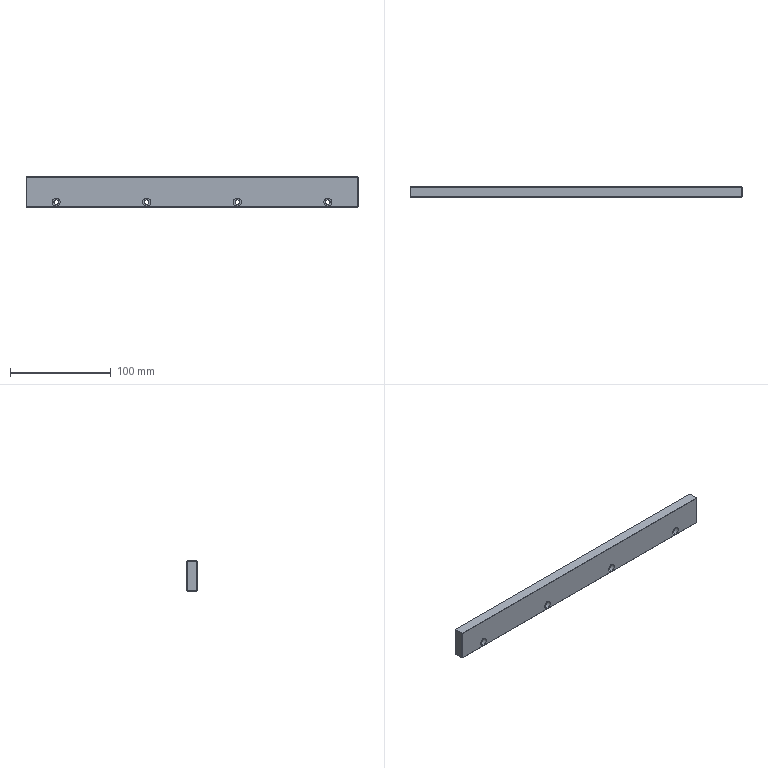Part | SolidWorks | features Chamfer 1, Extrusion 1, HoleWzd 1 | 1 solid | 46 faces | box 330 x 10 x 30 mm | volume 97693 mm3 | plane 30 | cylinder 16 | commonest cylinder face diameters 4.5 x8 8 x8
STEP:
#1=CARTESIAN_POINT('',(135.,4.4,-6.));
#2=VERTEX_POINT('',#1);
#3=CARTESIAN_POINT('',(135.,4.4,-14.));
#4=VERTEX_POINT('',#3);
#5=CARTESIAN_POINT('',(135.,4.4,-10.));
#6=DIRECTION('',(0.,-1.,0.));
#7=DIRECTION('',(0.,0.,-1.));
#8=AXIS2_PLACEMENT_3D('',#5,#6,#7);
#9=CIRCLE('',#8,4.);
#10=EDGE_CURVE('',#2,#4,#9,.T.);
#11=ORIENTED_EDGE('',*,*,#10,.F.);
#12=CARTESIAN_POINT('',(135.,0.,-6.));
#13=VERTEX_POINT('',#12);
#14=CARTESIAN_POINT('',(135.,0.,-6.));
#15=DIRECTION('',(0.,-1.,0.));
#16=VECTOR('',#15,1000.);
#17=LINE('',#14,#16);
#18=EDGE_CURVE('',#2,#13,#17,.T.);
#19=ORIENTED_EDGE('',*,*,#18,.T.);
#20=CARTESIAN_POINT('',(135.,0.,-14.));
#21=VERTEX_POINT('',#20);
#22=CARTESIAN_POINT('',(135.,0.,-10.));
#23=DIRECTION('',(0.,-1.,0.));
#24=DIRECTION('',(0.,0.,-1.));
#25=AXIS2_PLACEMENT_3D('',#22,#23,#24);
#26=CIRCLE('',#25,4.);
#27=EDGE_CURVE('',#13,#21,#26,.T.);
#28=ORIENTED_EDGE('',*,*,#27,.T.);
#29=CARTESIAN_POINT('',(135.,0.,-14.));
#30=DIRECTION('',(0.,-1.,0.));
#31=VECTOR('',#30,1000.);
#32=LINE('',#29,#31);
#33=EDGE_CURVE('',#4,#21,#32,.T.);
#34=ORIENTED_EDGE('',*,*,#33,.F.);
#35=EDGE_LOOP('',(#11,#19,#28,#34));
#36=FACE_OUTER_BOUND('',#35,.T.);
#37=CARTESIAN_POINT('',(135.,0.,-10.));
#38=DIRECTION('',(0.,-1.,0.));
#39=DIRECTION('',(0.,0.,-1.));
#40=AXIS2_PLACEMENT_3D('',#37,#38,#39);
#41=CYLINDRICAL_SURFACE('',#40,4.);
#42=ADVANCED_FACE('',(#36),#41,.F.);
#43=CARTESIAN_POINT('',(135.,10.,-7.75));
#44=VERTEX_POINT('',#43);
#45=CARTESIAN_POINT('',(135.,10.,-12.25));
#46=VERTEX_POINT('',#45);
#47=CARTESIAN_POINT('',(135.,10.,-10.));
#48=DIRECTION('',(0.,-1.,0.));
#49=DIRECTION('',(0.,0.,-1.));
#50=AXIS2_PLACEMENT_3D('',#47,#48,#49);
#51=CIRCLE('',#50,2.25);
#52=EDGE_CURVE('',#44,#46,#51,.T.);
#53=ORIENTED_EDGE('',*,*,#52,.F.);
#54=CARTESIAN_POINT('',(135.,4.4,-7.75));
#55=VERTEX_POINT('',#54);
#56=CARTESIAN_POINT('',(135.,0.,-7.75));
#57=DIRECTION('',(0.,-1.,0.));
#58=VECTOR('',#57,1000.);
#59=LINE('',#56,#58);
#60=EDGE_CURVE('',#44,#55,#59,.T.);
#61=ORIENTED_EDGE('',*,*,#60,.T.);
#62=CARTESIAN_POINT('',(135.,4.4,-12.25));
#63=VERTEX_POINT('',#62);
#64=CARTESIAN_POINT('',(135.,4.4,-10.));
#65=DIRECTION('',(0.,-1.,0.));
#66=DIRECTION('',(0.,0.,-1.));
#67=AXIS2_PLACEMENT_3D('',#64,#65,#66);
#68=CIRCLE('',#67,2.25);
#69=EDGE_CURVE('',#55,#63,#68,.T.);
#70=ORIENTED_EDGE('',*,*,#69,.T.);
#71=CARTESIAN_POINT('',(135.,0.,-12.25));
#72=DIRECTION('',(0.,-1.,0.));
#73=VECTOR('',#72,1000.);
#74=LINE('',#71,#73);
#75=EDGE_CURVE('',#46,#63,#74,.T.);
#76=ORIENTED_EDGE('',*,*,#75,.F.);
#77=EDGE_LOOP('',(#53,#61,#70,#76));
#78=FACE_OUTER_BOUND('',#77,.T.);
#79=CARTESIAN_POINT('',(135.,0.,-10.));
#80=DIRECTION('',(0.,-1.,0.));
#81=DIRECTION('',(0.,0.,-1.));
#82=AXIS2_PLACEMENT_3D('',#79,#80,#81);
#83=CYLINDRICAL_SURFACE('',#82,2.25);
#84=ADVANCED_FACE('',(#78),#83,.F.);
#85=CARTESIAN_POINT('',(45.,4.4,-6.));
#86=VERTEX_POINT('',#85);
#87=CARTESIAN_POINT('',(45.,4.4,-14.));
#88=VERTEX_POINT('',#87);
#89=CARTESIAN_POINT('',(45.,4.4,-10.));
#90=DIRECTION('',(0.,-1.,0.));
#91=DIRECTION('',(0.,0.,-1.));
#92=AXIS2_PLACEMENT_3D('',#89,#90,#91);
#93=CIRCLE('',#92,4.);
#94=EDGE_CURVE('',#86,#88,#93,.T.);
#95=ORIENTED_EDGE('',*,*,#94,.F.);
#96=CARTESIAN_POINT('',(45.,0.,-6.));
#97=VERTEX_POINT('',#96);
#98=CARTESIAN_POINT('',(45.,0.,-6.));
#99=DIRECTION('',(0.,-1.,0.));
#100=VECTOR('',#99,1000.);
#101=LINE('',#98,#100);
#102=EDGE_CURVE('',#86,#97,#101,.T.);
#103=ORIENTED_EDGE('',*,*,#102,.T.);
#104=CARTESIAN_POINT('',(45.,0.,-14.));
#105=VERTEX_POINT('',#104);
#106=CARTESIAN_POINT('',(45.,0.,-10.));
#107=DIRECTION('',(0.,-1.,0.));
#108=DIRECTION('',(0.,0.,-1.));
#109=AXIS2_PLACEMENT_3D('',#106,#107,#108);
#110=CIRCLE('',#109,4.);
#111=EDGE_CURVE('',#97,#105,#110,.T.);
#112=ORIENTED_EDGE('',*,*,#111,.T.);
#113=CARTESIAN_POINT('',(45.,0.,-14.));
#114=DIRECTION('',(0.,-1.,0.));
#115=VECTOR('',#114,1000.);
#116=LINE('',#113,#115);
#117=EDGE_CURVE('',#88,#105,#116,.T.);
#118=ORIENTED_EDGE('',*,*,#117,.F.);
#119=EDGE_LOOP('',(#95,#103,#112,#118));
#120=FACE_OUTER_BOUND('',#119,.T.);
#121=CARTESIAN_POINT('',(45.,0.,-10.));
#122=DIRECTION('',(0.,-1.,0.));
#123=DIRECTION('',(0.,0.,-1.));
#124=AXIS2_PLACEMENT_3D('',#121,#122,#123);
#125=CYLINDRICAL_SURFACE('',#124,4.);
#126=ADVANCED_FACE('',(#120),#125,.F.);
#127=CARTESIAN_POINT('',(45.,10.,-7.75));
#128=VERTEX_POINT('',#127);
#129=CARTESIAN_POINT('',(45.,10.,-12.25));
#130=VERTEX_POINT('',#129);
#131=CARTESIAN_POINT('',(45.,10.,-10.));
#132=DIRECTION('',(0.,-1.,0.));
#133=DIRECTION('',(0.,0.,-1.));
#134=AXIS2_PLACEMENT_3D('',#131,#132,#133);
#135=CIRCLE('',#134,2.25);
#136=EDGE_CURVE('',#128,#130,#135,.T.);
#137=ORIENTED_EDGE('',*,*,#136,.F.);
#138=CARTESIAN_POINT('',(45.,4.4,-7.75));
#139=VERTEX_POINT('',#138);
#140=CARTESIAN_POINT('',(45.,0.,-7.75));
#141=DIRECTION('',(0.,-1.,0.));
#142=VECTOR('',#141,1000.);
#143=LINE('',#140,#142);
#144=EDGE_CURVE('',#128,#139,#143,.T.);
#145=ORIENTED_EDGE('',*,*,#144,.T.);
#146=CARTESIAN_POINT('',(45.,4.4,-12.25));
#147=VERTEX_POINT('',#146);
#148=CARTESIAN_POINT('',(45.,4.4,-10.));
#149=DIRECTION('',(0.,-1.,0.));
#150=DIRECTION('',(0.,0.,-1.));
#151=AXIS2_PLACEMENT_3D('',#148,#149,#150);
#152=CIRCLE('',#151,2.25);
#153=EDGE_CURVE('',#139,#147,#152,.T.);
#154=ORIENTED_EDGE('',*,*,#153,.T.);
#155=CARTESIAN_POINT('',(45.,0.,-12.25));
#156=DIRECTION('',(0.,-1.,0.));
#157=VECTOR('',#156,1000.);
#158=LINE('',#155,#157);
#159=EDGE_CURVE('',#130,#147,#158,.T.);
#160=ORIENTED_EDGE('',*,*,#159,.F.);
#161=EDGE_LOOP('',(#137,#145,#154,#160));
#162=FACE_OUTER_BOUND('',#161,.T.);
#163=CARTESIAN_POINT('',(45.,0.,-10.));
#164=DIRECTION('',(0.,-1.,0.));
#165=DIRECTION('',(0.,0.,-1.));
#166=AXIS2_PLACEMENT_3D('',#163,#164,#165);
#167=CYLINDRICAL_SURFACE('',#166,2.25);
#168=ADVANCED_FACE('',(#162),#167,.F.);
#169=CARTESIAN_POINT('',(-45.,4.4,-6.));
#170=VERTEX_POINT('',#169);
#171=CARTESIAN_POINT('',(-45.,4.4,-14.));
#172=VERTEX_POINT('',#171);
#173=CARTESIAN_POINT('',(-45.,4.4,-10.));
#174=DIRECTION('',(0.,-1.,0.));
#175=DIRECTION('',(0.,0.,-1.));
#176=AXIS2_PLACEMENT_3D('',#173,#174,#175);
#177=CIRCLE('',#176,4.);
#178=EDGE_CURVE('',#170,#172,#177,.T.);
#179=ORIENTED_EDGE('',*,*,#178,.F.);
#180=CARTESIAN_POINT('',(-45.,0.,-6.));
#181=VERTEX_POINT('',#180);
#182=CARTESIAN_POINT('',(-45.,0.,-6.));
#183=DIRECTION('',(0.,-1.,0.));
#184=VECTOR('',#183,1000.);
#185=LINE('',#182,#184);
#186=EDGE_CURVE('',#170,#181,#185,.T.);
#187=ORIENTED_EDGE('',*,*,#186,.T.);
#188=CARTESIAN_POINT('',(-45.,0.,-14.));
#189=VERTEX_POINT('',#188);
#190=CARTESIAN_POINT('',(-45.,0.,-10.));
#191=DIRECTION('',(0.,-1.,0.));
#192=DIRECTION('',(0.,0.,-1.));
#193=AXIS2_PLACEMENT_3D('',#190,#191,#192);
#194=CIRCLE('',#193,4.);
#195=EDGE_CURVE('',#181,#189,#194,.T.);
#196=ORIENTED_EDGE('',*,*,#195,.T.);
#197=CARTESIAN_POINT('',(-45.,0.,-14.));
#198=DIRECTION('',(0.,-1.,0.));
#199=VECTOR('',#198,1000.);
#200=LINE('',#197,#199);
#201=EDGE_CURVE('',#172,#189,#200,.T.);
#202=ORIENTED_EDGE('',*,*,#201,.F.);
#203=EDGE_LOOP('',(#179,#187,#196,#202));
#204=FACE_OUTER_BOUND('',#203,.T.);
#205=CARTESIAN_POINT('',(-45.,0.,-10.));
#206=DIRECTION('',(0.,-1.,0.));
#207=DIRECTION('',(0.,0.,-1.));
#208=AXIS2_PLACEMENT_3D('',#205,#206,#207);
#209=CYLINDRICAL_SURFACE('',#208,4.);
#210=ADVANCED_FACE('',(#204),#209,.F.);
#211=CARTESIAN_POINT('',(-45.,10.,-7.75));
#212=VERTEX_POINT('',#211);
#213=CARTESIAN_POINT('',(-45.,10.,-12.25));
#214=VERTEX_POINT('',#213);
#215=CARTESIAN_POINT('',(-45.,10.,-10.));
#216=DIRECTION('',(0.,-1.,0.));
#217=DIRECTION('',(0.,0.,-1.));
#218=AXIS2_PLACEMENT_3D('',#215,#216,#217);
#219=CIRCLE('',#218,2.25);
#220=EDGE_CURVE('',#212,#214,#219,.T.);
#221=ORIENTED_EDGE('',*,*,#220,.F.);
#222=CARTESIAN_POINT('',(-45.,4.4,-7.75));
#223=VERTEX_POINT('',#222);
#224=CARTESIAN_POINT('',(-45.,0.,-7.75));
#225=DIRECTION('',(0.,-1.,0.));
#226=VECTOR('',#225,1000.);
#227=LINE('',#224,#226);
#228=EDGE_CURVE('',#212,#223,#227,.T.);
#229=ORIENTED_EDGE('',*,*,#228,.T.);
#230=CARTESIAN_POINT('',(-45.,4.4,-12.25));
#231=VERTEX_POINT('',#230);
#232=CARTESIAN_POINT('',(-45.,4.4,-10.));
#233=DIRECTION('',(0.,-1.,0.));
#234=DIRECTION('',(0.,0.,-1.));
#235=AXIS2_PLACEMENT_3D('',#232,#233,#234);
#236=CIRCLE('',#235,2.25);
#237=EDGE_CURVE('',#223,#231,#236,.T.);
#238=ORIENTED_EDGE('',*,*,#237,.T.);
#239=CARTESIAN_POINT('',(-45.,0.,-12.25));
#240=DIRECTION('',(0.,-1.,0.));
#241=VECTOR('',#240,1000.);
#242=LINE('',#239,#241);
#243=EDGE_CURVE('',#214,#231,#242,.T.);
#244=ORIENTED_EDGE('',*,*,#243,.F.);
#245=EDGE_LOOP('',(#221,#229,#238,#244));
#246=FACE_OUTER_BOUND('',#245,.T.);
#247=CARTESIAN_POINT('',(-45.,0.,-10.));
#248=DIRECTION('',(0.,-1.,0.));
#249=DIRECTION('',(0.,0.,-1.));
#250=AXIS2_PLACEMENT_3D('',#247,#248,#249);
#251=CYLINDRICAL_SURFACE('',#250,2.25);
#252=ADVANCED_FACE('',(#246),#251,.F.);
#253=CARTESIAN_POINT('',(-135.,4.4,-6.));
#254=VERTEX_POINT('',#253);
#255=CARTESIAN_POINT('',(-135.,4.4,-14.));
#256=VERTEX_POINT('',#255);
#257=CARTESIAN_POINT('',(-135.,4.4,-10.));
#258=DIRECTION('',(0.,-1.,0.));
#259=DIRECTION('',(0.,0.,-1.));
#260=AXIS2_PLACEMENT_3D('',#257,#258,#259);
#261=CIRCLE('',#260,4.);
#262=EDGE_CURVE('',#254,#256,#261,.T.);
#263=ORIENTED_EDGE('',*,*,#262,.F.);
#264=CARTESIAN_POINT('',(-135.,0.,-6.));
#265=VERTEX_POINT('',#264);
#266=CARTESIAN_POINT('',(-135.,0.,-6.));
#267=DIRECTION('',(0.,-1.,0.));
#268=VECTOR('',#267,1000.);
#269=LINE('',#266,#268);
#270=EDGE_CURVE('',#254,#265,#269,.T.);
#271=ORIENTED_EDGE('',*,*,#270,.T.);
#272=CARTESIAN_POINT('',(-135.,0.,-14.));
#273=VERTEX_POINT('',#272);
#274=CARTESIAN_POINT('',(-135.,0.,-10.));
#275=DIRECTION('',(0.,-1.,0.));
#276=DIRECTION('',(0.,0.,-1.));
#277=AXIS2_PLACEMENT_3D('',#274,#275,#276);
#278=CIRCLE('',#277,4.);
#279=EDGE_CURVE('',#265,#273,#278,.T.);
#280=ORIENTED_EDGE('',*,*,#279,.T.);
#281=CARTESIAN_POINT('',(-135.,0.,-14.));
#282=DIRECTION('',(0.,-1.,0.));
#283=VECTOR('',#282,1000.);
#284=LINE('',#281,#283);
#285=EDGE_CURVE('',#256,#273,#284,.T.);
#286=ORIENTED_EDGE('',*,*,#285,.F.);
#287=EDGE_LOOP('',(#263,#271,#280,#286));
#288=FACE_OUTER_BOUND('',#287,.T.);
#289=CARTESIAN_POINT('',(-135.,0.,-10.));
#290=DIRECTION('',(0.,-1.,0.));
#291=DIRECTION('',(0.,0.,-1.));
#292=AXIS2_PLACEMENT_3D('',#289,#290,#291);
#293=CYLINDRICAL_SURFACE('',#292,4.);
#294=ADVANCED_FACE('',(#288),#293,.F.);
#295=CARTESIAN_POINT('',(-135.,10.,-7.75));
#296=VERTEX_POINT('',#295);
#297=CARTESIAN_POINT('',(-135.,10.,-12.25));
#298=VERTEX_POINT('',#297);
#299=CARTESIAN_POINT('',(-135.,10.,-10.));
#300=DIRECTION('',(0.,-1.,0.));
#301=DIRECTION('',(0.,0.,-1.));
#302=AXIS2_PLACEMENT_3D('',#299,#300,#301);
#303=CIRCLE('',#302,2.25);
#304=EDGE_CURVE('',#296,#298,#303,.T.);
#305=ORIENTED_EDGE('',*,*,#304,.F.);
#306=CARTESIAN_POINT('',(-135.,4.4,-7.75));
#307=VERTEX_POINT('',#306);
#308=CARTESIAN_POINT('',(-135.,0.,-7.75));
#309=DIRECTION('',(0.,-1.,0.));
#310=VECTOR('',#309,1000.);
#311=LINE('',#308,#310);
#312=EDGE_CURVE('',#296,#307,#311,.T.);
#313=ORIENTED_EDGE('',*,*,#312,.T.);
#314=CARTESIAN_POINT('',(-135.,4.4,-12.25));
#315=VERTEX_POINT('',#314);
#316=CARTESIAN_POINT('',(-135.,4.4,-10.));
#317=DIRECTION('',(0.,-1.,0.));
#318=DIRECTION('',(0.,0.,-1.));
#319=AXIS2_PLACEMENT_3D('',#316,#317,#318);
#320=CIRCLE('',#319,2.25);
#321=EDGE_CURVE('',#307,#315,#320,.T.);
#322=ORIENTED_EDGE('',*,*,#321,.T.);
#323=CARTESIAN_POINT('',(-135.,0.,-12.25));
#324=DIRECTION('',(0.,-1.,0.));
#325=VECTOR('',#324,1000.);
#326=LINE('',#323,#325);
#327=EDGE_CURVE('',#298,#315,#326,.T.);
#328=ORIENTED_EDGE('',*,*,#327,.F.);
#329=EDGE_LOOP('',(#305,#313,#322,#328));
#330=FACE_OUTER_BOUND('',#329,.T.);
#331=CARTESIAN_POINT('',(-135.,0.,-10.));
#332=DIRECTION('',(0.,-1.,0.));
#333=DIRECTION('',(0.,0.,-1.));
#334=AXIS2_PLACEMENT_3D('',#331,#332,#333);
#335=CYLINDRICAL_SURFACE('',#334,2.25);
#336=ADVANCED_FACE('',(#330),#335,.F.);
#337=CARTESIAN_POINT('',(165.,9.7,-14.7));
#338=VERTEX_POINT('',#337);
#339=CARTESIAN_POINT('',(165.,9.7,14.7));
#340=VERTEX_POINT('',#339);
#341=CARTESIAN_POINT('',(165.,9.7,15.));
#342=DIRECTION('',(0.,0.,1.));
#343=VECTOR('',#342,1000.);
#344=LINE('',#341,#343);
#345=EDGE_CURVE('',#338,#340,#344,.T.);
#346=ORIENTED_EDGE('',*,*,#345,.T.);
#347=CARTESIAN_POINT('',(165.,0.3,14.7));
#348=VERTEX_POINT('',#347);
#349=CARTESIAN_POINT('',(165.,10.,14.7));
#350=DIRECTION('',(0.,-1.,0.));
#351=VECTOR('',#350,1000.);
#352=LINE('',#349,#351);
#353=EDGE_CURVE('',#340,#348,#352,.T.);
#354=ORIENTED_EDGE('',*,*,#353,.T.);
#355=CARTESIAN_POINT('',(165.,0.3,-14.7));
#356=VERTEX_POINT('',#355);
#357=CARTESIAN_POINT('',(165.,0.3,-15.));
#358=DIRECTION('',(0.,0.,-1.));
#359=VECTOR('',#358,1000.);
#360=LINE('',#357,#359);
#361=EDGE_CURVE('',#348,#356,#360,.T.);
#362=ORIENTED_EDGE('',*,*,#361,.T.);
#363=CARTESIAN_POINT('',(165.,10.,-14.7));
#364=DIRECTION('',(0.,1.,0.));
#365=VECTOR('',#364,1000.);
#366=LINE('',#363,#365);
#367=EDGE_CURVE('',#356,#338,#366,.T.);
#368=ORIENTED_EDGE('',*,*,#367,.T.);
#369=EDGE_LOOP('',(#346,#354,#362,#368));
#370=FACE_OUTER_BOUND('',#369,.T.);
#371=CARTESIAN_POINT('',(165.,10.,-15.));
#372=DIRECTION('',(-1.,0.,0.));
#373=DIRECTION('',(0.,0.,1.));
#374=AXIS2_PLACEMENT_3D('',#371,#372,#373);
#375=PLANE('',#374);
#376=ADVANCED_FACE('',(#370),#375,.F.);
#377=CARTESIAN_POINT('',(-164.7,9.7,-15.));
#378=VERTEX_POINT('',#377);
#379=CARTESIAN_POINT('',(164.7,9.7,-15.));
#380=VERTEX_POINT('',#379);
#381=CARTESIAN_POINT('',(165.,9.7,-15.));
#382=DIRECTION('',(1.,0.,0.));
#383=VECTOR('',#382,1000.);
#384=LINE('',#381,#383);
#385=EDGE_CURVE('',#378,#380,#384,.T.);
#386=ORIENTED_EDGE('',*,*,#385,.T.);
#387=CARTESIAN_POINT('',(164.7,0.3,-15.));
#388=VERTEX_POINT('',#387);
#389=CARTESIAN_POINT('',(164.7,10.,-15.));
#390=DIRECTION('',(0.,-1.,0.));
#391=VECTOR('',#390,1000.);
#392=LINE('',#389,#391);
#393=EDGE_CURVE('',#380,#388,#392,.T.);
#394=ORIENTED_EDGE('',*,*,#393,.T.);
#395=CARTESIAN_POINT('',(-164.7,0.3,-15.));
#396=VERTEX_POINT('',#395);
#397=CARTESIAN_POINT('',(-165.,0.3,-15.));
#398=DIRECTION('',(-1.,0.,0.));
#399=VECTOR('',#398,1000.);
#400=LINE('',#397,#399);
#401=EDGE_CURVE('',#388,#396,#400,.T.);
#402=ORIENTED_EDGE('',*,*,#401,.T.);
#403=CARTESIAN_POINT('',(-164.7,10.,-15.));
#404=DIRECTION('',(0.,1.,0.));
#405=VECTOR('',#404,1000.);
#406=LINE('',#403,#405);
#407=EDGE_CURVE('',#396,#378,#406,.T.);
#408=ORIENTED_EDGE('',*,*,#407,.T.);
#409=EDGE_LOOP('',(#386,#394,#402,#408));
#410=FACE_OUTER_BOUND('',#409,.T.);
#411=CARTESIAN_POINT('',(-165.,10.,-15.));
#412=DIRECTION('',(0.,0.,1.));
#413=DIRECTION('',(1.,0.,0.));
#414=AXIS2_PLACEMENT_3D('',#411,#412,#413);
#415=PLANE('',#414);
#416=ADVANCED_FACE('',(#410),#415,.F.);
#417=CARTESIAN_POINT('',(-165.,0.3,14.7));
#418=VERTEX_POINT('',#417);
#419=CARTESIAN_POINT('',(-165.,9.7,14.7));
#420=VERTEX_POINT('',#419);
#421=CARTESIAN_POINT('',(-165.,10.,14.7));
#422=DIRECTION('',(0.,1.,0.));
#423=VECTOR('',#422,1000.);
#424=LINE('',#421,#423);
#425=EDGE_CURVE('',#418,#420,#424,.T.);
#426=ORIENTED_EDGE('',*,*,#425,.T.);
#427=CARTESIAN_POINT('',(-165.,9.7,-14.7));
#428=VERTEX_POINT('',#427);
#429=CARTESIAN_POINT('',(-165.,9.7,-15.));
#430=DIRECTION('',(0.,0.,-1.));
#431=VECTOR('',#430,1000.);
#432=LINE('',#429,#431);
#433=EDGE_CURVE('',#420,#428,#432,.T.);
#434=ORIENTED_EDGE('',*,*,#433,.T.);
#435=CARTESIAN_POINT('',(-165.,0.3,-14.7));
#436=VERTEX_POINT('',#435);
#437=CARTESIAN_POINT('',(-165.,10.,-14.7));
#438=DIRECTION('',(0.,-1.,0.));
#439=VECTOR('',#438,1000.);
#440=LINE('',#437,#439);
#441=EDGE_CURVE('',#428,#436,#440,.T.);
#442=ORIENTED_EDGE('',*,*,#441,.T.);
#443=CARTESIAN_POINT('',(-165.,0.3,-15.));
#444=DIRECTION('',(0.,0.,1.));
#445=VECTOR('',#444,1000.);
#446=LINE('',#443,#445);
#447=EDGE_CURVE('',#436,#418,#446,.T.);
#448=ORIENTED_EDGE('',*,*,#447,.T.);
#449=EDGE_LOOP('',(#426,#434,#442,#448));
#450=FACE_OUTER_BOUND('',#449,.T.);
#451=CARTESIAN_POINT('',(-165.,10.,-15.));
#452=DIRECTION('',(1.,0.,0.));
#453=DIRECTION('',(0.,0.,-1.));
#454=AXIS2_PLACEMENT_3D('',#451,#452,#453);
#455=PLANE('',#454);
#456=ADVANCED_FACE('',(#450),#455,.F.);
#457=CARTESIAN_POINT('',(164.7,0.3,15.));
#458=VERTEX_POINT('',#457);
#459=CARTESIAN_POINT('',(164.7,9.7,15.));
#460=VERTEX_POINT('',#459);
#461=CARTESIAN_POINT('',(164.7,10.,15.));
#462=DIRECTION('',(0.,1.,0.));
#463=VECTOR('',#462,1000.);
#464=LINE('',#461,#463);
#465=EDGE_CURVE('',#458,#460,#464,.T.);
#466=ORIENTED_EDGE('',*,*,#465,.T.);
#467=CARTESIAN_POINT('',(-164.7,9.7,15.));
#468=VERTEX_POINT('',#467);
#469=CARTESIAN_POINT('',(-165.,9.7,15.));
#470=DIRECTION('',(-1.,0.,0.));
#471=VECTOR('',#470,1000.);
#472=LINE('',#469,#471);
#473=EDGE_CURVE('',#460,#468,#472,.T.);
#474=ORIENTED_EDGE('',*,*,#473,.T.);
#475=CARTESIAN_POINT('',(-164.7,0.3,15.));
#476=VERTEX_POINT('',#475);
#477=CARTESIAN_POINT('',(-164.7,10.,15.));
#478=DIRECTION('',(0.,-1.,0.));
#479=VECTOR('',#478,1000.);
#480=LINE('',#477,#479);
#481=EDGE_CURVE('',#468,#476,#480,.T.);
#482=ORIENTED_EDGE('',*,*,#481,.T.);
#483=CARTESIAN_POINT('',(-165.,0.3,15.));
#484=DIRECTION('',(1.,0.,0.));
#485=VECTOR('',#484,1000.);
#486=LINE('',#483,#485);
#487=EDGE_CURVE('',#476,#458,#486,.T.);
#488=ORIENTED_EDGE('',*,*,#487,.T.);
#489=EDGE_LOOP('',(#466,#474,#482,#488));
#490=FACE_OUTER_BOUND('',#489,.T.);
#491=CARTESIAN_POINT('',(-165.,10.,15.));
#492=DIRECTION('',(0.,0.,-1.));
#493=DIRECTION('',(-1.,0.,0.));
#494=AXIS2_PLACEMENT_3D('',#491,#492,#493);
#495=PLANE('',#494);
#496=ADVANCED_FACE('',(#490),#495,.F.);
#497=CARTESIAN_POINT('',(-164.7,10.,14.7));
#498=VERTEX_POINT('',#497);
#499=CARTESIAN_POINT('',(164.7,10.,14.7));
#500=VERTEX_POINT('',#499);
#501=CARTESIAN_POINT('',(165.,10.,14.7));
#502=DIRECTION('',(1.,0.,0.));
#503=VECTOR('',#502,1000.);
#504=LINE('',#501,#503);
#505=EDGE_CURVE('',#498,#500,#504,.T.);
#506=ORIENTED_EDGE('',*,*,#505,.T.);
#507=CARTESIAN_POINT('',(164.7,10.,-14.7));
#508=VERTEX_POINT('',#507);
#509=CARTESIAN_POINT('',(164.7,10.,-15.));
#510=DIRECTION('',(0.,0.,-1.));
#511=VECTOR('',#510,1000.);
#512=LINE('',#509,#511);
#513=EDGE_CURVE('',#500,#508,#512,.T.);
#514=ORIENTED_EDGE('',*,*,#513,.T.);
#515=CARTESIAN_POINT('',(-164.7,10.,-14.7));
#516=VERTEX_POINT('',#515);
#517=CARTESIAN_POINT('',(-165.,10.,-14.7));
#518=DIRECTION('',(-1.,0.,0.));
#519=VECTOR('',#518,1000.);
#520=LINE('',#517,#519);
#521=EDGE_CURVE('',#508,#516,#520,.T.);
#522=ORIENTED_EDGE('',*,*,#521,.T.);
#523=CARTESIAN_POINT('',(-164.7,10.,15.));
#524=DIRECTION('',(0.,0.,1.));
#525=VECTOR('',#524,1000.);
#526=LINE('',#523,#525);
#527=EDGE_CURVE('',#516,#498,#526,.T.);
#528=ORIENTED_EDGE('',*,*,#527,.T.);
#529=EDGE_LOOP('',(#506,#514,#522,#528));
#530=FACE_OUTER_BOUND('',#529,.T.);
#531=CARTESIAN_POINT('',(135.,10.,-10.));
#532=DIRECTION('',(0.,-1.,0.));
#533=DIRECTION('',(0.,0.,-1.));
#534=AXIS2_PLACEMENT_3D('',#531,#532,#533);
#535=CIRCLE('',#534,2.25);
#536=EDGE_CURVE('',#46,#44,#535,.T.);
#537=ORIENTED_EDGE('',*,*,#536,.T.);
#538=ORIENTED_EDGE('',*,*,#52,.T.);
#539=EDGE_LOOP('',(#537,#538));
#540=FACE_BOUND('',#539,.T.);
#541=CARTESIAN_POINT('',(45.,10.,-10.));
#542=DIRECTION('',(0.,-1.,0.));
#543=DIRECTION('',(0.,0.,-1.));
#544=AXIS2_PLACEMENT_3D('',#541,#542,#543);
#545=CIRCLE('',#544,2.25);
#546=EDGE_CURVE('',#130,#128,#545,.T.);
#547=ORIENTED_EDGE('',*,*,#546,.T.);
#548=ORIENTED_EDGE('',*,*,#136,.T.);
#549=EDGE_LOOP('',(#547,#548));
#550=FACE_BOUND('',#549,.T.);
#551=CARTESIAN_POINT('',(-45.,10.,-10.));
#552=DIRECTION('',(0.,-1.,0.));
#553=DIRECTION('',(0.,0.,-1.));
#554=AXIS2_PLACEMENT_3D('',#551,#552,#553);
#555=CIRCLE('',#554,2.25);
#556=EDGE_CURVE('',#214,#212,#555,.T.);
#557=ORIENTED_EDGE('',*,*,#556,.T.);
#558=ORIENTED_EDGE('',*,*,#220,.T.);
#559=EDGE_LOOP('',(#557,#558));
#560=FACE_BOUND('',#559,.T.);
#561=CARTESIAN_POINT('',(-135.,10.,-10.));
#562=DIRECTION('',(0.,-1.,0.));
#563=DIRECTION('',(0.,0.,-1.));
#564=AXIS2_PLACEMENT_3D('',#561,#562,#563);
#565=CIRCLE('',#564,2.25);
#566=EDGE_CURVE('',#298,#296,#565,.T.);
#567=ORIENTED_EDGE('',*,*,#566,.T.);
#568=ORIENTED_EDGE('',*,*,#304,.T.);
#569=EDGE_LOOP('',(#567,#568));
#570=FACE_BOUND('',#569,.T.);
#571=CARTESIAN_POINT('',(0.,10.,0.));
#572=DIRECTION('',(0.,1.,0.));
#573=DIRECTION('',(0.,0.,1.));
#574=AXIS2_PLACEMENT_3D('',#571,#572,#573);
#575=PLANE('',#574);
#576=ADVANCED_FACE('',(#530,#540,#550,#560,#570),#575,.T.);
#577=CARTESIAN_POINT('',(-164.7,0.,-14.7));
#578=VERTEX_POINT('',#577);
#579=CARTESIAN_POINT('',(164.7,0.,-14.7));
#580=VERTEX_POINT('',#579);
#581=CARTESIAN_POINT('',(0.,0.,-14.7));
#582=DIRECTION('',(1.,0.,0.));
#583=VECTOR('',#582,1000.);
#584=LINE('',#581,#583);
#585=EDGE_CURVE('',#578,#580,#584,.T.);
#586=ORIENTED_EDGE('',*,*,#585,.T.);
#587=CARTESIAN_POINT('',(164.7,0.,14.7));
#588=VERTEX_POINT('',#587);
#589=CARTESIAN_POINT('',(164.7,0.,0.));
#590=DIRECTION('',(0.,0.,1.));
#591=VECTOR('',#590,1000.);
#592=LINE('',#589,#591);
#593=EDGE_CURVE('',#580,#588,#592,.T.);
#594=ORIENTED_EDGE('',*,*,#593,.T.);
#595=CARTESIAN_POINT('',(-164.7,0.,14.7));
#596=VERTEX_POINT('',#595);
#597=CARTESIAN_POINT('',(0.,0.,14.7));
#598=DIRECTION('',(-1.,0.,0.));
#599=VECTOR('',#598,1000.);
#600=LINE('',#597,#599);
#601=EDGE_CURVE('',#588,#596,#600,.T.);
#602=ORIENTED_EDGE('',*,*,#601,.T.);
#603=CARTESIAN_POINT('',(-164.7,0.,0.));
#604=DIRECTION('',(0.,0.,-1.));
#605=VECTOR('',#604,1000.);
#606=LINE('',#603,#605);
#607=EDGE_CURVE('',#596,#578,#606,.T.);
#608=ORIENTED_EDGE('',*,*,#607,.T.);
#609=EDGE_LOOP('',(#586,#594,#602,#608));
#610=FACE_OUTER_BOUND('',#609,.T.);
#611=CARTESIAN_POINT('',(135.,0.,-10.));
#612=DIRECTION('',(0.,-1.,0.));
#613=DIRECTION('',(0.,0.,-1.));
#614=AXIS2_PLACEMENT_3D('',#611,#612,#613);
#615=CIRCLE('',#614,4.);
#616=EDGE_CURVE('',#21,#13,#615,.T.);
#617=ORIENTED_EDGE('',*,*,#616,.F.);
#618=ORIENTED_EDGE('',*,*,#27,.F.);
#619=EDGE_LOOP('',(#617,#618));
#620=FACE_BOUND('',#619,.T.);
#621=CARTESIAN_POINT('',(45.,0.,-10.));
#622=DIRECTION('',(0.,-1.,0.));
#623=DIRECTION('',(0.,0.,-1.));
#624=AXIS2_PLACEMENT_3D('',#621,#622,#623);
#625=CIRCLE('',#624,4.);
#626=EDGE_CURVE('',#105,#97,#625,.T.);
#627=ORIENTED_EDGE('',*,*,#626,.F.);
#628=ORIENTED_EDGE('',*,*,#111,.F.);
#629=EDGE_LOOP('',(#627,#628));
#630=FACE_BOUND('',#629,.T.);
#631=CARTESIAN_POINT('',(-45.,0.,-10.));
#632=DIRECTION('',(0.,-1.,0.));
#633=DIRECTION('',(0.,0.,-1.));
#634=AXIS2_PLACEMENT_3D('',#631,#632,#633);
#635=CIRCLE('',#634,4.);
#636=EDGE_CURVE('',#189,#181,#635,.T.);
#637=ORIENTED_EDGE('',*,*,#636,.F.);
#638=ORIENTED_EDGE('',*,*,#195,.F.);
#639=EDGE_LOOP('',(#637,#638));
#640=FACE_BOUND('',#639,.T.);
#641=CARTESIAN_POINT('',(-135.,0.,-10.));
#642=DIRECTION('',(0.,-1.,0.));
#643=DIRECTION('',(0.,0.,-1.));
#644=AXIS2_PLACEMENT_3D('',#641,#642,#643);
#645=CIRCLE('',#644,4.);
#646=EDGE_CURVE('',#273,#265,#645,.T.);
#647=ORIENTED_EDGE('',*,*,#646,.F.);
#648=ORIENTED_EDGE('',*,*,#279,.F.);
#649=EDGE_LOOP('',(#647,#648));
#650=FACE_BOUND('',#649,.T.);
#651=CARTESIAN_POINT('',(0.,0.,0.));
#652=DIRECTION('',(0.,1.,0.));
#653=DIRECTION('',(0.,0.,1.));
#654=AXIS2_PLACEMENT_3D('',#651,#652,#653);
#655=PLANE('',#654);
#656=ADVANCED_FACE('',(#610,#620,#630,#640,#650),#655,.F.);
#657=ORIENTED_EDGE('',*,*,#312,.F.);
#658=ORIENTED_EDGE('',*,*,#566,.F.);
#659=ORIENTED_EDGE('',*,*,#327,.T.);
#660=CARTESIAN_POINT('',(-135.,4.4,-10.));
#661=DIRECTION('',(0.,-1.,0.));
#662=DIRECTION('',(0.,0.,-1.));
#663=AXIS2_PLACEMENT_3D('',#660,#661,#662);
#664=CIRCLE('',#663,2.25);
#665=EDGE_CURVE('',#315,#307,#664,.T.);
#666=ORIENTED_EDGE('',*,*,#665,.T.);
#667=EDGE_LOOP('',(#657,#658,#659,#666));
#668=FACE_OUTER_BOUND('',#667,.T.);
#669=CARTESIAN_POINT('',(-135.,0.,-10.));
#670=DIRECTION('',(0.,-1.,0.));
#671=DIRECTION('',(0.,0.,-1.));
#672=AXIS2_PLACEMENT_3D('',#669,#670,#671);
#673=CYLINDRICAL_SURFACE('',#672,2.25);
#674=ADVANCED_FACE('',(#668),#673,.F.);
#675=ORIENTED_EDGE('',*,*,#665,.F.);
#676=ORIENTED_EDGE('',*,*,#321,.F.);
#677=EDGE_LOOP('',(#675,#676));
#678=FACE_BOUND('',#677,.T.);
#679=CARTESIAN_POINT('',(-135.,4.4,-10.));
#680=DIRECTION('',(0.,-1.,0.));
#681=DIRECTION('',(0.,0.,-1.));
#682=AXIS2_PLACEMENT_3D('',#679,#680,#681);
#683=CIRCLE('',#682,4.);
#684=EDGE_CURVE('',#256,#254,#683,.T.);
#685=ORIENTED_EDGE('',*,*,#684,.T.);
#686=ORIENTED_EDGE('',*,*,#262,.T.);
#687=EDGE_LOOP('',(#685,#686));
#688=FACE_OUTER_BOUND('',#687,.T.);
#689=CARTESIAN_POINT('',(-132.75,4.4,-10.));
#690=DIRECTION('',(0.,1.,0.));
#691=DIRECTION('',(0.,0.,1.));
#692=AXIS2_PLACEMENT_3D('',#689,#690,#691);
#693=PLANE('',#692);
#694=ADVANCED_FACE('',(#678,#688),#693,.F.);
#695=ORIENTED_EDGE('',*,*,#270,.F.);
#696=ORIENTED_EDGE('',*,*,#684,.F.);
#697=ORIENTED_EDGE('',*,*,#285,.T.);
#698=ORIENTED_EDGE('',*,*,#646,.T.);
#699=EDGE_LOOP('',(#695,#696,#697,#698));
#700=FACE_OUTER_BOUND('',#699,.T.);
#701=CARTESIAN_POINT('',(-135.,0.,-10.));
#702=DIRECTION('',(0.,-1.,0.));
#703=DIRECTION('',(0.,0.,-1.));
#704=AXIS2_PLACEMENT_3D('',#701,#702,#703);
#705=CYLINDRICAL_SURFACE('',#704,4.);
#706=ADVANCED_FACE('',(#700),#705,.F.);
#707=ORIENTED_EDGE('',*,*,#228,.F.);
#708=ORIENTED_EDGE('',*,*,#556,.F.);
#709=ORIENTED_EDGE('',*,*,#243,.T.);
#710=CARTESIAN_POINT('',(-45.,4.4,-10.));
#711=DIRECTION('',(0.,-1.,0.));
#712=DIRECTION('',(0.,0.,-1.));
#713=AXIS2_PLACEMENT_3D('',#710,#711,#712);
#714=CIRCLE('',#713,2.25);
#715=EDGE_CURVE('',#231,#223,#714,.T.);
#716=ORIENTED_EDGE('',*,*,#715,.T.);
#717=EDGE_LOOP('',(#707,#708,#709,#716));
#718=FACE_OUTER_BOUND('',#717,.T.);
#719=CARTESIAN_POINT('',(-45.,0.,-10.));
#720=DIRECTION('',(0.,-1.,0.));
#721=DIRECTION('',(0.,0.,-1.));
#722=AXIS2_PLACEMENT_3D('',#719,#720,#721);
#723=CYLINDRICAL_SURFACE('',#722,2.25);
#724=ADVANCED_FACE('',(#718),#723,.F.);
#725=ORIENTED_EDGE('',*,*,#715,.F.);
#726=ORIENTED_EDGE('',*,*,#237,.F.);
#727=EDGE_LOOP('',(#725,#726));
#728=FACE_BOUND('',#727,.T.);
#729=CARTESIAN_POINT('',(-45.,4.4,-10.));
#730=DIRECTION('',(0.,-1.,0.));
#731=DIRECTION('',(0.,0.,-1.));
#732=AXIS2_PLACEMENT_3D('',#729,#730,#731);
#733=CIRCLE('',#732,4.);
#734=EDGE_CURVE('',#172,#170,#733,.T.);
#735=ORIENTED_EDGE('',*,*,#734,.T.);
#736=ORIENTED_EDGE('',*,*,#178,.T.);
#737=EDGE_LOOP('',(#735,#736));
#738=FACE_OUTER_BOUND('',#737,.T.);
#739=CARTESIAN_POINT('',(-42.75,4.4,-10.));
#740=DIRECTION('',(0.,1.,0.));
#741=DIRECTION('',(0.,0.,1.));
#742=AXIS2_PLACEMENT_3D('',#739,#740,#741);
#743=PLANE('',#742);
#744=ADVANCED_FACE('',(#728,#738),#743,.F.);
#745=ORIENTED_EDGE('',*,*,#186,.F.);
#746=ORIENTED_EDGE('',*,*,#734,.F.);
#747=ORIENTED_EDGE('',*,*,#201,.T.);
#748=ORIENTED_EDGE('',*,*,#636,.T.);
#749=EDGE_LOOP('',(#745,#746,#747,#748));
#750=FACE_OUTER_BOUND('',#749,.T.);
#751=CARTESIAN_POINT('',(-45.,0.,-10.));
#752=DIRECTION('',(0.,-1.,0.));
#753=DIRECTION('',(0.,0.,-1.));
#754=AXIS2_PLACEMENT_3D('',#751,#752,#753);
#755=CYLINDRICAL_SURFACE('',#754,4.);
#756=ADVANCED_FACE('',(#750),#755,.F.);
#757=ORIENTED_EDGE('',*,*,#144,.F.);
#758=ORIENTED_EDGE('',*,*,#546,.F.);
#759=ORIENTED_EDGE('',*,*,#159,.T.);
#760=CARTESIAN_POINT('',(45.,4.4,-10.));
#761=DIRECTION('',(0.,-1.,0.));
#762=DIRECTION('',(0.,0.,-1.));
#763=AXIS2_PLACEMENT_3D('',#760,#761,#762);
#764=CIRCLE('',#763,2.25);
#765=EDGE_CURVE('',#147,#139,#764,.T.);
#766=ORIENTED_EDGE('',*,*,#765,.T.);
#767=EDGE_LOOP('',(#757,#758,#759,#766));
#768=FACE_OUTER_BOUND('',#767,.T.);
#769=CARTESIAN_POINT('',(45.,0.,-10.));
#770=DIRECTION('',(0.,-1.,0.));
#771=DIRECTION('',(0.,0.,-1.));
#772=AXIS2_PLACEMENT_3D('',#769,#770,#771);
#773=CYLINDRICAL_SURFACE('',#772,2.25);
#774=ADVANCED_FACE('',(#768),#773,.F.);
#775=ORIENTED_EDGE('',*,*,#765,.F.);
#776=ORIENTED_EDGE('',*,*,#153,.F.);
#777=EDGE_LOOP('',(#775,#776));
#778=FACE_BOUND('',#777,.T.);
#779=CARTESIAN_POINT('',(45.,4.4,-10.));
#780=DIRECTION('',(0.,-1.,0.));
#781=DIRECTION('',(0.,0.,-1.));
#782=AXIS2_PLACEMENT_3D('',#779,#780,#781);
#783=CIRCLE('',#782,4.);
#784=EDGE_CURVE('',#88,#86,#783,.T.);
#785=ORIENTED_EDGE('',*,*,#784,.T.);
#786=ORIENTED_EDGE('',*,*,#94,.T.);
#787=EDGE_LOOP('',(#785,#786));
#788=FACE_OUTER_BOUND('',#787,.T.);
#789=CARTESIAN_POINT('',(47.25,4.4,-10.));
#790=DIRECTION('',(0.,1.,0.));
#791=DIRECTION('',(0.,0.,1.));
#792=AXIS2_PLACEMENT_3D('',#789,#790,#791);
#793=PLANE('',#792);
#794=ADVANCED_FACE('',(#778,#788),#793,.F.);
#795=ORIENTED_EDGE('',*,*,#102,.F.);
#796=ORIENTED_EDGE('',*,*,#784,.F.);
#797=ORIENTED_EDGE('',*,*,#117,.T.);
#798=ORIENTED_EDGE('',*,*,#626,.T.);
#799=EDGE_LOOP('',(#795,#796,#797,#798));
#800=FACE_OUTER_BOUND('',#799,.T.);
#801=CARTESIAN_POINT('',(45.,0.,-10.));
#802=DIRECTION('',(0.,-1.,0.));
#803=DIRECTION('',(0.,0.,-1.));
#804=AXIS2_PLACEMENT_3D('',#801,#802,#803);
#805=CYLINDRICAL_SURFACE('',#804,4.);
#806=ADVANCED_FACE('',(#800),#805,.F.);
#807=ORIENTED_EDGE('',*,*,#60,.F.);
#808=ORIENTED_EDGE('',*,*,#536,.F.);
#809=ORIENTED_EDGE('',*,*,#75,.T.);
#810=CARTESIAN_POINT('',(135.,4.4,-10.));
#811=DIRECTION('',(0.,-1.,0.));
#812=DIRECTION('',(0.,0.,-1.));
#813=AXIS2_PLACEMENT_3D('',#810,#811,#812);
#814=CIRCLE('',#813,2.25);
#815=EDGE_CURVE('',#63,#55,#814,.T.);
#816=ORIENTED_EDGE('',*,*,#815,.T.);
#817=EDGE_LOOP('',(#807,#808,#809,#816));
#818=FACE_OUTER_BOUND('',#817,.T.);
#819=CARTESIAN_POINT('',(135.,0.,-10.));
#820=DIRECTION('',(0.,-1.,0.));
#821=DIRECTION('',(0.,0.,-1.));
#822=AXIS2_PLACEMENT_3D('',#819,#820,#821);
#823=CYLINDRICAL_SURFACE('',#822,2.25);
#824=ADVANCED_FACE('',(#818),#823,.F.);
#825=ORIENTED_EDGE('',*,*,#815,.F.);
#826=ORIENTED_EDGE('',*,*,#69,.F.);
#827=EDGE_LOOP('',(#825,#826));
#828=FACE_BOUND('',#827,.T.);
#829=CARTESIAN_POINT('',(135.,4.4,-10.));
#830=DIRECTION('',(0.,-1.,0.));
#831=DIRECTION('',(0.,0.,-1.));
#832=AXIS2_PLACEMENT_3D('',#829,#830,#831);
#833=CIRCLE('',#832,4.);
#834=EDGE_CURVE('',#4,#2,#833,.T.);
#835=ORIENTED_EDGE('',*,*,#834,.T.);
#836=ORIENTED_EDGE('',*,*,#10,.T.);
#837=EDGE_LOOP('',(#835,#836));
#838=FACE_OUTER_BOUND('',#837,.T.);
#839=CARTESIAN_POINT('',(137.25,4.4,-10.));
#840=DIRECTION('',(0.,1.,0.));
#841=DIRECTION('',(0.,0.,1.));
#842=AXIS2_PLACEMENT_3D('',#839,#840,#841);
#843=PLANE('',#842);
#844=ADVANCED_FACE('',(#828,#838),#843,.F.);
#845=ORIENTED_EDGE('',*,*,#18,.F.);
#846=ORIENTED_EDGE('',*,*,#834,.F.);
#847=ORIENTED_EDGE('',*,*,#33,.T.);
#848=ORIENTED_EDGE('',*,*,#616,.T.);
#849=EDGE_LOOP('',(#845,#846,#847,#848));
#850=FACE_OUTER_BOUND('',#849,.T.);
#851=CARTESIAN_POINT('',(135.,0.,-10.));
#852=DIRECTION('',(0.,-1.,0.));
#853=DIRECTION('',(0.,0.,-1.));
#854=AXIS2_PLACEMENT_3D('',#851,#852,#853);
#855=CYLINDRICAL_SURFACE('',#854,4.);
#856=ADVANCED_FACE('',(#850),#855,.F.);
#857=CARTESIAN_POINT('',(-164.7,0.,14.7));
#858=DIRECTION('',(0.7071,-0.7071,0.));
#859=VECTOR('',#858,1000.);
#860=LINE('',#857,#859);
#861=EDGE_CURVE('',#418,#596,#860,.T.);
#862=ORIENTED_EDGE('',*,*,#861,.F.);
#863=ORIENTED_EDGE('',*,*,#447,.F.);
#864=CARTESIAN_POINT('',(-164.7,0.,-14.7));
#865=DIRECTION('',(-0.7071,0.7071,0.));
#866=VECTOR('',#865,1000.);
#867=LINE('',#864,#866);
#868=EDGE_CURVE('',#578,#436,#867,.T.);
#869=ORIENTED_EDGE('',*,*,#868,.F.);
#870=ORIENTED_EDGE('',*,*,#607,.F.);
#871=EDGE_LOOP('',(#862,#863,#869,#870));
#872=FACE_OUTER_BOUND('',#871,.T.);
#873=CARTESIAN_POINT('',(-165.,0.3,-15.));
#874=DIRECTION('',(0.7071,0.7071,0.));
#875=DIRECTION('',(0.,0.,1.));
#876=AXIS2_PLACEMENT_3D('',#873,#874,#875);
#877=PLANE('',#876);
#878=ADVANCED_FACE('',(#872),#877,.F.);
#879=CARTESIAN_POINT('',(-164.85,0.3,14.85));
#880=DIRECTION('',(0.7071,0.,0.7071));
#881=VECTOR('',#880,1000.);
#882=LINE('',#879,#881);
#883=EDGE_CURVE('',#418,#476,#882,.T.);
#884=ORIENTED_EDGE('',*,*,#883,.F.);
#885=ORIENTED_EDGE('',*,*,#861,.T.);
#886=CARTESIAN_POINT('',(-164.7,0.,14.7));
#887=DIRECTION('',(0.,-0.7071,-0.7071));
#888=VECTOR('',#887,1000.);
#889=LINE('',#886,#888);
#890=EDGE_CURVE('',#476,#596,#889,.T.);
#891=ORIENTED_EDGE('',*,*,#890,.F.);
#892=EDGE_LOOP('',(#884,#885,#891));
#893=FACE_OUTER_BOUND('',#892,.T.);
#894=CARTESIAN_POINT('',(-164.7,0.,14.7));
#895=DIRECTION('',(-0.5774,-0.5774,0.5774));
#896=DIRECTION('',(0.7071,-0.7071,0.));
#897=AXIS2_PLACEMENT_3D('',#894,#895,#896);
#898=PLANE('',#897);
#899=ADVANCED_FACE('',(#893),#898,.T.);
#900=CARTESIAN_POINT('',(-164.7,0.,-14.7));
#901=DIRECTION('',(0.,0.7071,-0.7071));
#902=VECTOR('',#901,1000.);
#903=LINE('',#900,#902);
#904=EDGE_CURVE('',#578,#396,#903,.T.);
#905=ORIENTED_EDGE('',*,*,#904,.F.);
#906=ORIENTED_EDGE('',*,*,#868,.T.);
#907=CARTESIAN_POINT('',(-164.85,0.3,-14.85));
#908=DIRECTION('',(-0.7071,0.,0.7071));
#909=VECTOR('',#908,1000.);
#910=LINE('',#907,#909);
#911=EDGE_CURVE('',#396,#436,#910,.T.);
#912=ORIENTED_EDGE('',*,*,#911,.F.);
#913=EDGE_LOOP('',(#905,#906,#912));
#914=FACE_OUTER_BOUND('',#913,.T.);
#915=CARTESIAN_POINT('',(-164.7,0.,-14.7));
#916=DIRECTION('',(-0.5774,-0.5774,-0.5774));
#917=DIRECTION('',(0.7071,-0.7071,0.));
#918=AXIS2_PLACEMENT_3D('',#915,#916,#917);
#919=PLANE('',#918);
#920=ADVANCED_FACE('',(#914),#919,.T.);
#921=ORIENTED_EDGE('',*,*,#890,.T.);
#922=ORIENTED_EDGE('',*,*,#601,.F.);
#923=CARTESIAN_POINT('',(164.7,0.,14.7));
#924=DIRECTION('',(0.,-0.7071,-0.7071));
#925=VECTOR('',#924,1000.);
#926=LINE('',#923,#925);
#927=EDGE_CURVE('',#458,#588,#926,.T.);
#928=ORIENTED_EDGE('',*,*,#927,.F.);
#929=ORIENTED_EDGE('',*,*,#487,.F.);
#930=EDGE_LOOP('',(#921,#922,#928,#929));
#931=FACE_OUTER_BOUND('',#930,.T.);
#932=CARTESIAN_POINT('',(-165.,0.3,15.));
#933=DIRECTION('',(0.,0.7071,-0.7071));
#934=DIRECTION('',(1.,0.,0.));
#935=AXIS2_PLACEMENT_3D('',#932,#933,#934);
#936=PLANE('',#935);
#937=ADVANCED_FACE('',(#931),#936,.F.);
#938=ORIENTED_EDGE('',*,*,#883,.T.);
#939=ORIENTED_EDGE('',*,*,#481,.F.);
#940=CARTESIAN_POINT('',(-164.7,9.7,15.));
#941=DIRECTION('',(0.7071,0.,0.7071));
#942=VECTOR('',#941,1000.);
#943=LINE('',#940,#942);
#944=EDGE_CURVE('',#420,#468,#943,.T.);
#945=ORIENTED_EDGE('',*,*,#944,.F.);
#946=ORIENTED_EDGE('',*,*,#425,.F.);
#947=EDGE_LOOP('',(#938,#939,#945,#946));
#948=FACE_OUTER_BOUND('',#947,.T.);
#949=CARTESIAN_POINT('',(-164.7,10.,15.));
#950=DIRECTION('',(0.7071,0.,-0.7071));
#951=DIRECTION('',(0.,-1.,0.));
#952=AXIS2_PLACEMENT_3D('',#949,#950,#951);
#953=PLANE('',#952);
#954=ADVANCED_FACE('',(#948),#953,.F.);
#955=CARTESIAN_POINT('',(-165.,9.7,-14.7));
#956=DIRECTION('',(0.7071,0.7071,0.));
#957=VECTOR('',#956,1000.);
#958=LINE('',#955,#957);
#959=EDGE_CURVE('',#428,#516,#958,.T.);
#960=ORIENTED_EDGE('',*,*,#959,.F.);
#961=ORIENTED_EDGE('',*,*,#433,.F.);
#962=CARTESIAN_POINT('',(-164.85,9.85,14.7));
#963=DIRECTION('',(-0.7071,-0.7071,0.));
#964=VECTOR('',#963,1000.);
#965=LINE('',#962,#964);
#966=EDGE_CURVE('',#498,#420,#965,.T.);
#967=ORIENTED_EDGE('',*,*,#966,.F.);
#968=ORIENTED_EDGE('',*,*,#527,.F.);
#969=EDGE_LOOP('',(#960,#961,#967,#968));
#970=FACE_OUTER_BOUND('',#969,.T.);
#971=CARTESIAN_POINT('',(-164.7,10.,0.));
#972=DIRECTION('',(-0.7071,0.7071,0.));
#973=DIRECTION('',(0.,0.,-1.));
#974=AXIS2_PLACEMENT_3D('',#971,#972,#973);
#975=PLANE('',#974);
#976=ADVANCED_FACE('',(#970),#975,.T.);
#977=ORIENTED_EDGE('',*,*,#911,.T.);
#978=ORIENTED_EDGE('',*,*,#441,.F.);
#979=CARTESIAN_POINT('',(-165.,9.7,-14.7));
#980=DIRECTION('',(-0.7071,0.,0.7071));
#981=VECTOR('',#980,1000.);
#982=LINE('',#979,#981);
#983=EDGE_CURVE('',#378,#428,#982,.T.);
#984=ORIENTED_EDGE('',*,*,#983,.F.);
#985=ORIENTED_EDGE('',*,*,#407,.F.);
#986=EDGE_LOOP('',(#977,#978,#984,#985));
#987=FACE_OUTER_BOUND('',#986,.T.);
#988=CARTESIAN_POINT('',(-165.,10.,-14.7));
#989=DIRECTION('',(0.7071,0.,0.7071));
#990=DIRECTION('',(0.,-1.,0.));
#991=AXIS2_PLACEMENT_3D('',#988,#989,#990);
#992=PLANE('',#991);
#993=ADVANCED_FACE('',(#987),#992,.F.);
#994=ORIENTED_EDGE('',*,*,#904,.T.);
#995=ORIENTED_EDGE('',*,*,#401,.F.);
#996=CARTESIAN_POINT('',(164.7,0.15,-14.85));
#997=DIRECTION('',(0.,0.7071,-0.7071));
#998=VECTOR('',#997,1000.);
#999=LINE('',#996,#998);
#1000=EDGE_CURVE('',#580,#388,#999,.T.);
#1001=ORIENTED_EDGE('',*,*,#1000,.F.);
#1002=ORIENTED_EDGE('',*,*,#585,.F.);
#1003=EDGE_LOOP('',(#994,#995,#1001,#1002));
#1004=FACE_OUTER_BOUND('',#1003,.T.);
#1005=CARTESIAN_POINT('',(-165.,0.3,-15.));
#1006=DIRECTION('',(0.,0.7071,0.7071));
#1007=DIRECTION('',(-1.,0.,0.));
#1008=AXIS2_PLACEMENT_3D('',#1005,#1006,#1007);
#1009=PLANE('',#1008);
#1010=ADVANCED_FACE('',(#1004),#1009,.F.);
#1011=CARTESIAN_POINT('',(164.7,0.,14.7));
#1012=DIRECTION('',(0.7071,0.7071,0.));
#1013=VECTOR('',#1012,1000.);
#1014=LINE('',#1011,#1013);
#1015=EDGE_CURVE('',#588,#348,#1014,.T.);
#1016=ORIENTED_EDGE('',*,*,#1015,.F.);
#1017=ORIENTED_EDGE('',*,*,#593,.F.);
#1018=CARTESIAN_POINT('',(165.,0.3,-14.7));
#1019=DIRECTION('',(-0.7071,-0.7071,0.));
#1020=VECTOR('',#1019,1000.);
#1021=LINE('',#1018,#1020);
#1022=EDGE_CURVE('',#356,#580,#1021,.T.);
#1023=ORIENTED_EDGE('',*,*,#1022,.F.);
#1024=ORIENTED_EDGE('',*,*,#361,.F.);
#1025=EDGE_LOOP('',(#1016,#1017,#1023,#1024));
#1026=FACE_OUTER_BOUND('',#1025,.T.);
#1027=CARTESIAN_POINT('',(165.,0.3,-15.));
#1028=DIRECTION('',(-0.7071,0.7071,0.));
#1029=DIRECTION('',(0.,0.,-1.));
#1030=AXIS2_PLACEMENT_3D('',#1027,#1028,#1029);
#1031=PLANE('',#1030);
#1032=ADVANCED_FACE('',(#1026),#1031,.F.);
#1033=ORIENTED_EDGE('',*,*,#927,.T.);
#1034=ORIENTED_EDGE('',*,*,#1015,.T.);
#1035=CARTESIAN_POINT('',(164.85,0.3,14.85));
#1036=DIRECTION('',(0.7071,0.,-0.7071));
#1037=VECTOR('',#1036,1000.);
#1038=LINE('',#1035,#1037);
#1039=EDGE_CURVE('',#458,#348,#1038,.T.);
#1040=ORIENTED_EDGE('',*,*,#1039,.F.);
#1041=EDGE_LOOP('',(#1033,#1034,#1040));
#1042=FACE_OUTER_BOUND('',#1041,.T.);
#1043=CARTESIAN_POINT('',(164.7,0.,14.7));
#1044=DIRECTION('',(0.5774,-0.5774,0.5774));
#1045=DIRECTION('',(0.,-0.7071,-0.7071));
#1046=AXIS2_PLACEMENT_3D('',#1043,#1044,#1045);
#1047=PLANE('',#1046);
#1048=ADVANCED_FACE('',(#1042),#1047,.T.);
#1049=ORIENTED_EDGE('',*,*,#966,.T.);
#1050=ORIENTED_EDGE('',*,*,#944,.T.);
#1051=CARTESIAN_POINT('',(-164.7,9.7,15.));
#1052=DIRECTION('',(0.,-0.7071,0.7071));
#1053=VECTOR('',#1052,1000.);
#1054=LINE('',#1051,#1053);
#1055=EDGE_CURVE('',#498,#468,#1054,.T.);
#1056=ORIENTED_EDGE('',*,*,#1055,.F.);
#1057=EDGE_LOOP('',(#1049,#1050,#1056));
#1058=FACE_OUTER_BOUND('',#1057,.T.);
#1059=CARTESIAN_POINT('',(-164.7,9.7,15.));
#1060=DIRECTION('',(-0.5774,0.5774,0.5774));
#1061=DIRECTION('',(0.7071,0.,0.7071));
#1062=AXIS2_PLACEMENT_3D('',#1059,#1060,#1061);
#1063=PLANE('',#1062);
#1064=ADVANCED_FACE('',(#1058),#1063,.T.);
#1065=ORIENTED_EDGE('',*,*,#983,.T.);
#1066=ORIENTED_EDGE('',*,*,#959,.T.);
#1067=CARTESIAN_POINT('',(-164.7,9.85,-14.85));
#1068=DIRECTION('',(0.,0.7071,0.7071));
#1069=VECTOR('',#1068,1000.);
#1070=LINE('',#1067,#1069);
#1071=EDGE_CURVE('',#378,#516,#1070,.T.);
#1072=ORIENTED_EDGE('',*,*,#1071,.F.);
#1073=EDGE_LOOP('',(#1065,#1066,#1072));
#1074=FACE_OUTER_BOUND('',#1073,.T.);
#1075=CARTESIAN_POINT('',(-165.,9.7,-14.7));
#1076=DIRECTION('',(-0.5774,0.5774,-0.5774));
#1077=DIRECTION('',(-0.7071,-0.7071,0.));
#1078=AXIS2_PLACEMENT_3D('',#1075,#1076,#1077);
#1079=PLANE('',#1078);
#1080=ADVANCED_FACE('',(#1074),#1079,.T.);
#1081=ORIENTED_EDGE('',*,*,#1022,.T.);
#1082=ORIENTED_EDGE('',*,*,#1000,.T.);
#1083=CARTESIAN_POINT('',(165.,0.3,-14.7));
#1084=DIRECTION('',(-0.7071,0.,-0.7071));
#1085=VECTOR('',#1084,1000.);
#1086=LINE('',#1083,#1085);
#1087=EDGE_CURVE('',#356,#388,#1086,.T.);
#1088=ORIENTED_EDGE('',*,*,#1087,.F.);
#1089=EDGE_LOOP('',(#1081,#1082,#1088));
#1090=FACE_OUTER_BOUND('',#1089,.T.);
#1091=CARTESIAN_POINT('',(165.,0.3,-14.7));
#1092=DIRECTION('',(0.5774,-0.5774,-0.5774));
#1093=DIRECTION('',(0.7071,0.7071,0.));
#1094=AXIS2_PLACEMENT_3D('',#1091,#1092,#1093);
#1095=PLANE('',#1094);
#1096=ADVANCED_FACE('',(#1090),#1095,.T.);
#1097=ORIENTED_EDGE('',*,*,#1039,.T.);
#1098=ORIENTED_EDGE('',*,*,#353,.F.);
#1099=CARTESIAN_POINT('',(165.,9.7,14.7));
#1100=DIRECTION('',(0.7071,0.,-0.7071));
#1101=VECTOR('',#1100,1000.);
#1102=LINE('',#1099,#1101);
#1103=EDGE_CURVE('',#460,#340,#1102,.T.);
#1104=ORIENTED_EDGE('',*,*,#1103,.F.);
#1105=ORIENTED_EDGE('',*,*,#465,.F.);
#1106=EDGE_LOOP('',(#1097,#1098,#1104,#1105));
#1107=FACE_OUTER_BOUND('',#1106,.T.);
#1108=CARTESIAN_POINT('',(165.,10.,14.7));
#1109=DIRECTION('',(-0.7071,0.,-0.7071));
#1110=DIRECTION('',(0.,-1.,0.));
#1111=AXIS2_PLACEMENT_3D('',#1108,#1109,#1110);
#1112=PLANE('',#1111);
#1113=ADVANCED_FACE('',(#1107),#1112,.F.);
#1114=ORIENTED_EDGE('',*,*,#1055,.T.);
#1115=ORIENTED_EDGE('',*,*,#473,.F.);
#1116=CARTESIAN_POINT('',(164.7,9.85,14.85));
#1117=DIRECTION('',(0.,-0.7071,0.7071));
#1118=VECTOR('',#1117,1000.);
#1119=LINE('',#1116,#1118);
#1120=EDGE_CURVE('',#500,#460,#1119,.T.);
#1121=ORIENTED_EDGE('',*,*,#1120,.F.);
#1122=ORIENTED_EDGE('',*,*,#505,.F.);
#1123=EDGE_LOOP('',(#1114,#1115,#1121,#1122));
#1124=FACE_OUTER_BOUND('',#1123,.T.);
#1125=CARTESIAN_POINT('',(0.,10.,14.7));
#1126=DIRECTION('',(0.,0.7071,0.7071));
#1127=DIRECTION('',(-1.,0.,0.));
#1128=AXIS2_PLACEMENT_3D('',#1125,#1126,#1127);
#1129=PLANE('',#1128);
#1130=ADVANCED_FACE('',(#1124),#1129,.T.);
#1131=ORIENTED_EDGE('',*,*,#1071,.T.);
#1132=ORIENTED_EDGE('',*,*,#521,.F.);
#1133=CARTESIAN_POINT('',(164.7,10.,-14.7));
#1134=DIRECTION('',(0.,0.7071,0.7071));
#1135=VECTOR('',#1134,1000.);
#1136=LINE('',#1133,#1135);
#1137=EDGE_CURVE('',#380,#508,#1136,.T.);
#1138=ORIENTED_EDGE('',*,*,#1137,.F.);
#1139=ORIENTED_EDGE('',*,*,#385,.F.);
#1140=EDGE_LOOP('',(#1131,#1132,#1138,#1139));
#1141=FACE_OUTER_BOUND('',#1140,.T.);
#1142=CARTESIAN_POINT('',(0.,10.,-14.7));
#1143=DIRECTION('',(0.,0.7071,-0.7071));
#1144=DIRECTION('',(1.,0.,0.));
#1145=AXIS2_PLACEMENT_3D('',#1142,#1143,#1144);
#1146=PLANE('',#1145);
#1147=ADVANCED_FACE('',(#1141),#1146,.T.);
#1148=ORIENTED_EDGE('',*,*,#1087,.T.);
#1149=ORIENTED_EDGE('',*,*,#393,.F.);
#1150=CARTESIAN_POINT('',(164.85,9.7,-14.85));
#1151=DIRECTION('',(-0.7071,0.,-0.7071));
#1152=VECTOR('',#1151,1000.);
#1153=LINE('',#1150,#1152);
#1154=EDGE_CURVE('',#338,#380,#1153,.T.);
#1155=ORIENTED_EDGE('',*,*,#1154,.F.);
#1156=ORIENTED_EDGE('',*,*,#367,.F.);
#1157=EDGE_LOOP('',(#1148,#1149,#1155,#1156));
#1158=FACE_OUTER_BOUND('',#1157,.T.);
#1159=CARTESIAN_POINT('',(164.7,10.,-15.));
#1160=DIRECTION('',(-0.7071,0.,0.7071));
#1161=DIRECTION('',(0.,-1.,0.));
#1162=AXIS2_PLACEMENT_3D('',#1159,#1160,#1161);
#1163=PLANE('',#1162);
#1164=ADVANCED_FACE('',(#1158),#1163,.F.);
#1165=ORIENTED_EDGE('',*,*,#1120,.T.);
#1166=ORIENTED_EDGE('',*,*,#1103,.T.);
#1167=CARTESIAN_POINT('',(165.,9.7,14.7));
#1168=DIRECTION('',(0.7071,-0.7071,0.));
#1169=VECTOR('',#1168,1000.);
#1170=LINE('',#1167,#1169);
#1171=EDGE_CURVE('',#500,#340,#1170,.T.);
#1172=ORIENTED_EDGE('',*,*,#1171,.F.);
#1173=EDGE_LOOP('',(#1165,#1166,#1172));
#1174=FACE_OUTER_BOUND('',#1173,.T.);
#1175=CARTESIAN_POINT('',(165.,9.7,14.7));
#1176=DIRECTION('',(0.5774,0.5774,0.5774));
#1177=DIRECTION('',(0.7071,0.,-0.7071));
#1178=AXIS2_PLACEMENT_3D('',#1175,#1176,#1177);
#1179=PLANE('',#1178);
#1180=ADVANCED_FACE('',(#1174),#1179,.T.);
#1181=ORIENTED_EDGE('',*,*,#1154,.T.);
#1182=ORIENTED_EDGE('',*,*,#1137,.T.);
#1183=CARTESIAN_POINT('',(164.7,10.,-14.7));
#1184=DIRECTION('',(-0.7071,0.7071,0.));
#1185=VECTOR('',#1184,1000.);
#1186=LINE('',#1183,#1185);
#1187=EDGE_CURVE('',#338,#508,#1186,.T.);
#1188=ORIENTED_EDGE('',*,*,#1187,.F.);
#1189=EDGE_LOOP('',(#1181,#1182,#1188));
#1190=FACE_OUTER_BOUND('',#1189,.T.);
#1191=CARTESIAN_POINT('',(164.7,10.,-14.7));
#1192=DIRECTION('',(0.5774,0.5774,-0.5774));
#1193=DIRECTION('',(-0.7071,0.7071,0.));
#1194=AXIS2_PLACEMENT_3D('',#1191,#1192,#1193);
#1195=PLANE('',#1194);
#1196=ADVANCED_FACE('',(#1190),#1195,.T.);
#1197=ORIENTED_EDGE('',*,*,#1171,.T.);
#1198=ORIENTED_EDGE('',*,*,#345,.F.);
#1199=ORIENTED_EDGE('',*,*,#1187,.T.);
#1200=ORIENTED_EDGE('',*,*,#513,.F.);
#1201=EDGE_LOOP('',(#1197,#1198,#1199,#1200));
#1202=FACE_OUTER_BOUND('',#1201,.T.);
#1203=CARTESIAN_POINT('',(164.7,10.,0.));
#1204=DIRECTION('',(0.7071,0.7071,0.));
#1205=DIRECTION('',(0.,0.,1.));
#1206=AXIS2_PLACEMENT_3D('',#1203,#1204,#1205);
#1207=PLANE('',#1206);
#1208=ADVANCED_FACE('',(#1202),#1207,.T.);
#1209=CLOSED_SHELL('',(#42,#84,#126,#168,#210,#252,#294,#336,#376,#416,#456,#496,#576,#656,#674,#694,#706,#724,#744,#756,#774,#794,#806,#824,#844,#856,#878,#899,#920,#937,#954,#976,#993,#1010,#1032,#1048,#1064,#1080,#1096,#1113,#1130,#1147,#1164,#1180,#1196,#1208));
#1210=MANIFOLD_SOLID_BREP('',#1209);
#1211=CARTESIAN_POINT('',(0.,0.,0.));
#1212=DIRECTION('',(0.,0.,1.));
#1213=DIRECTION('',(1.,0.,0.));
#1214=AXIS2_PLACEMENT_3D('',#1211,#1212,#1213);
#1215=(LENGTH_UNIT()NAMED_UNIT(*)SI_UNIT(.MILLI.,.METRE.));
#1216=UNCERTAINTY_MEASURE_WITH_UNIT(LENGTH_MEASURE(0.00001),#1215,'','');
#1217=(NAMED_UNIT(*)PLANE_ANGLE_UNIT()SI_UNIT($,.RADIAN.));
#1218=(NAMED_UNIT(*)SI_UNIT($,.STERADIAN.)SOLID_ANGLE_UNIT());
#1219=(GEOMETRIC_REPRESENTATION_CONTEXT(3)GLOBAL_UNCERTAINTY_ASSIGNED_CONTEXT((#1216))GLOBAL_UNIT_ASSIGNED_CONTEXT((#1215,#1217,#1218))REPRESENTATION_CONTEXT('',''));
#1220=ADVANCED_BREP_SHAPE_REPRESENTATION('',(#1210,#1214),#1219);